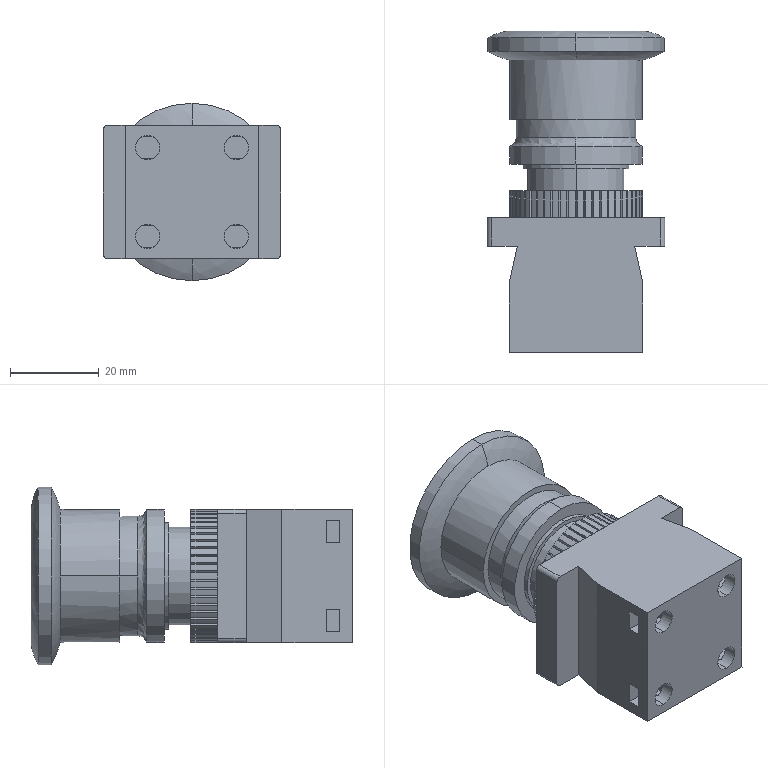Part | SolidWorks | features BaseBody 1 | 1 solid | 254 faces | box 40 x 72.5 x 40 mm | volume 57928 mm3 | plane 167 | cylinder 81 | spline 6 | commonest cylinder face diameters 30 x55 5.5 x8 22 x5 2 x4 26 x3 24 x2